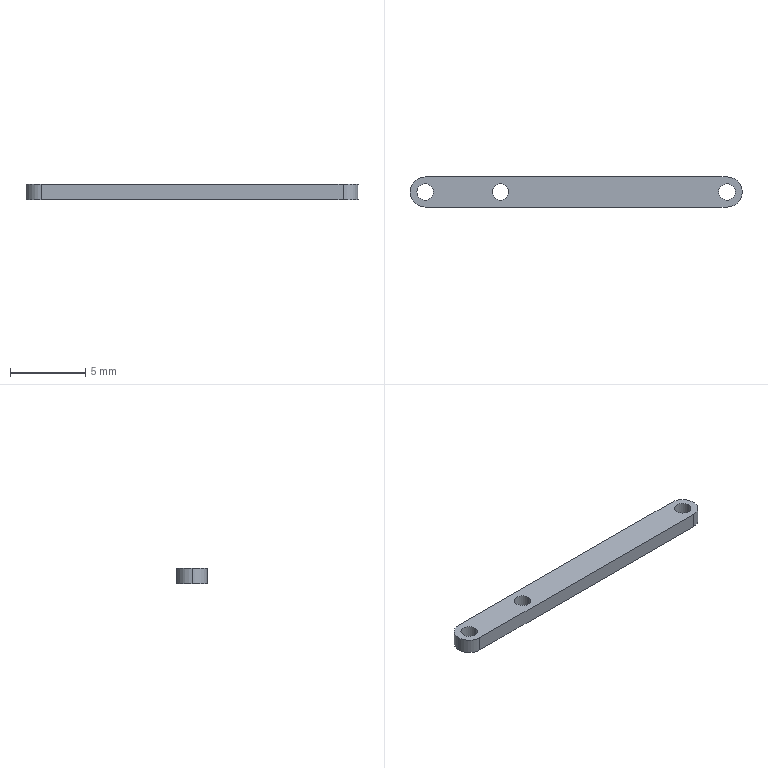Part | SolidWorks | features Extrusion 1, ICE 1 | 1 solid | 13 faces | box 22 x 2 x 1 mm | volume 40.291 mm3 | cylinder 9 | plane 4 | commonest cylinder face diameters 1.1 x6 2 x3
STEP:
#1=CARTESIAN_POINT('',(-5.55,0.,0.5));
#2=VERTEX_POINT('',#1);
#3=CARTESIAN_POINT('',(-4.45,0.,0.5));
#4=VERTEX_POINT('',#3);
#5=CARTESIAN_POINT('',(-5.,0.,0.5));
#6=DIRECTION('',(0.,0.,1.));
#7=DIRECTION('',(1.,0.,0.));
#8=AXIS2_PLACEMENT_3D('',#5,#6,#7);
#9=CIRCLE('',#8,0.55);
#10=EDGE_CURVE('',#2,#4,#9,.T.);
#11=ORIENTED_EDGE('',*,*,#10,.T.);
#12=CARTESIAN_POINT('',(-4.45,0.,-0.5));
#13=VERTEX_POINT('',#12);
#14=CARTESIAN_POINT('',(-4.45,0.,0.5));
#15=DIRECTION('',(0.,0.,-1.));
#16=VECTOR('',#15,1000.);
#17=LINE('',#14,#16);
#18=EDGE_CURVE('',#4,#13,#17,.T.);
#19=ORIENTED_EDGE('',*,*,#18,.T.);
#20=CARTESIAN_POINT('',(-5.55,0.,-0.5));
#21=VERTEX_POINT('',#20);
#22=CARTESIAN_POINT('',(-5.,0.,-0.5));
#23=DIRECTION('',(0.,0.,1.));
#24=DIRECTION('',(1.,0.,0.));
#25=AXIS2_PLACEMENT_3D('',#22,#23,#24);
#26=CIRCLE('',#25,0.55);
#27=EDGE_CURVE('',#21,#13,#26,.T.);
#28=ORIENTED_EDGE('',*,*,#27,.F.);
#29=CARTESIAN_POINT('',(-5.55,0.,0.5));
#30=DIRECTION('',(0.,0.,-1.));
#31=VECTOR('',#30,1000.);
#32=LINE('',#29,#31);
#33=EDGE_CURVE('',#2,#21,#32,.T.);
#34=ORIENTED_EDGE('',*,*,#33,.F.);
#35=EDGE_LOOP('',(#11,#19,#28,#34));
#36=FACE_OUTER_BOUND('',#35,.T.);
#37=CARTESIAN_POINT('',(-5.,0.,0.5));
#38=DIRECTION('',(0.,0.,-1.));
#39=DIRECTION('',(-1.,0.,0.));
#40=AXIS2_PLACEMENT_3D('',#37,#38,#39);
#41=CYLINDRICAL_SURFACE('',#40,0.55);
#42=ADVANCED_FACE('',(#36),#41,.F.);
#43=CARTESIAN_POINT('',(9.45,0.,0.5));
#44=VERTEX_POINT('',#43);
#45=CARTESIAN_POINT('',(10.55,0.,0.5));
#46=VERTEX_POINT('',#45);
#47=CARTESIAN_POINT('',(10.,0.,0.5));
#48=DIRECTION('',(0.,0.,1.));
#49=DIRECTION('',(1.,0.,0.));
#50=AXIS2_PLACEMENT_3D('',#47,#48,#49);
#51=CIRCLE('',#50,0.55);
#52=EDGE_CURVE('',#44,#46,#51,.T.);
#53=ORIENTED_EDGE('',*,*,#52,.T.);
#54=CARTESIAN_POINT('',(10.55,0.,-0.5));
#55=VERTEX_POINT('',#54);
#56=CARTESIAN_POINT('',(10.55,0.,0.5));
#57=DIRECTION('',(0.,0.,-1.));
#58=VECTOR('',#57,1000.);
#59=LINE('',#56,#58);
#60=EDGE_CURVE('',#46,#55,#59,.T.);
#61=ORIENTED_EDGE('',*,*,#60,.T.);
#62=CARTESIAN_POINT('',(9.45,0.,-0.5));
#63=VERTEX_POINT('',#62);
#64=CARTESIAN_POINT('',(10.,0.,-0.5));
#65=DIRECTION('',(0.,0.,1.));
#66=DIRECTION('',(1.,0.,0.));
#67=AXIS2_PLACEMENT_3D('',#64,#65,#66);
#68=CIRCLE('',#67,0.55);
#69=EDGE_CURVE('',#63,#55,#68,.T.);
#70=ORIENTED_EDGE('',*,*,#69,.F.);
#71=CARTESIAN_POINT('',(9.45,0.,0.5));
#72=DIRECTION('',(0.,0.,-1.));
#73=VECTOR('',#72,1000.);
#74=LINE('',#71,#73);
#75=EDGE_CURVE('',#44,#63,#74,.T.);
#76=ORIENTED_EDGE('',*,*,#75,.F.);
#77=EDGE_LOOP('',(#53,#61,#70,#76));
#78=FACE_OUTER_BOUND('',#77,.T.);
#79=CARTESIAN_POINT('',(10.,0.,0.5));
#80=DIRECTION('',(0.,0.,-1.));
#81=DIRECTION('',(-1.,0.,0.));
#82=AXIS2_PLACEMENT_3D('',#79,#80,#81);
#83=CYLINDRICAL_SURFACE('',#82,0.55);
#84=ADVANCED_FACE('',(#78),#83,.F.);
#85=CARTESIAN_POINT('',(-10.55,0.,0.5));
#86=VERTEX_POINT('',#85);
#87=CARTESIAN_POINT('',(-9.45,0.,0.5));
#88=VERTEX_POINT('',#87);
#89=CARTESIAN_POINT('',(-10.,0.,0.5));
#90=DIRECTION('',(0.,0.,1.));
#91=DIRECTION('',(1.,0.,0.));
#92=AXIS2_PLACEMENT_3D('',#89,#90,#91);
#93=CIRCLE('',#92,0.55);
#94=EDGE_CURVE('',#86,#88,#93,.T.);
#95=ORIENTED_EDGE('',*,*,#94,.T.);
#96=CARTESIAN_POINT('',(-9.45,0.,-0.5));
#97=VERTEX_POINT('',#96);
#98=CARTESIAN_POINT('',(-9.45,0.,0.5));
#99=DIRECTION('',(0.,0.,-1.));
#100=VECTOR('',#99,1000.);
#101=LINE('',#98,#100);
#102=EDGE_CURVE('',#88,#97,#101,.T.);
#103=ORIENTED_EDGE('',*,*,#102,.T.);
#104=CARTESIAN_POINT('',(-10.55,0.,-0.5));
#105=VERTEX_POINT('',#104);
#106=CARTESIAN_POINT('',(-10.,0.,-0.5));
#107=DIRECTION('',(0.,0.,1.));
#108=DIRECTION('',(1.,0.,0.));
#109=AXIS2_PLACEMENT_3D('',#106,#107,#108);
#110=CIRCLE('',#109,0.55);
#111=EDGE_CURVE('',#105,#97,#110,.T.);
#112=ORIENTED_EDGE('',*,*,#111,.F.);
#113=CARTESIAN_POINT('',(-10.55,0.,0.5));
#114=DIRECTION('',(0.,0.,-1.));
#115=VECTOR('',#114,1000.);
#116=LINE('',#113,#115);
#117=EDGE_CURVE('',#86,#105,#116,.T.);
#118=ORIENTED_EDGE('',*,*,#117,.F.);
#119=EDGE_LOOP('',(#95,#103,#112,#118));
#120=FACE_OUTER_BOUND('',#119,.T.);
#121=CARTESIAN_POINT('',(-10.,0.,0.5));
#122=DIRECTION('',(0.,0.,-1.));
#123=DIRECTION('',(-1.,0.,0.));
#124=AXIS2_PLACEMENT_3D('',#121,#122,#123);
#125=CYLINDRICAL_SURFACE('',#124,0.55);
#126=ADVANCED_FACE('',(#120),#125,.F.);
#127=CARTESIAN_POINT('',(-11.,0.,0.5));
#128=VERTEX_POINT('',#127);
#129=CARTESIAN_POINT('',(-10.,-1.,0.5));
#130=VERTEX_POINT('',#129);
#131=CARTESIAN_POINT('',(-10.,0.,0.5));
#132=DIRECTION('',(0.,0.,1.));
#133=DIRECTION('',(1.,0.,0.));
#134=AXIS2_PLACEMENT_3D('',#131,#132,#133);
#135=CIRCLE('',#134,1.);
#136=EDGE_CURVE('',#128,#130,#135,.T.);
#137=ORIENTED_EDGE('',*,*,#136,.F.);
#138=CARTESIAN_POINT('',(-11.,0.,-0.5));
#139=VERTEX_POINT('',#138);
#140=CARTESIAN_POINT('',(-11.,0.,0.5));
#141=DIRECTION('',(0.,0.,-1.));
#142=VECTOR('',#141,1000.);
#143=LINE('',#140,#142);
#144=EDGE_CURVE('',#128,#139,#143,.T.);
#145=ORIENTED_EDGE('',*,*,#144,.T.);
#146=CARTESIAN_POINT('',(-10.,-1.,-0.5));
#147=VERTEX_POINT('',#146);
#148=CARTESIAN_POINT('',(-10.,0.,-0.5));
#149=DIRECTION('',(0.,0.,1.));
#150=DIRECTION('',(1.,0.,0.));
#151=AXIS2_PLACEMENT_3D('',#148,#149,#150);
#152=CIRCLE('',#151,1.);
#153=EDGE_CURVE('',#139,#147,#152,.T.);
#154=ORIENTED_EDGE('',*,*,#153,.T.);
#155=CARTESIAN_POINT('',(-10.,-1.,0.5));
#156=DIRECTION('',(0.,0.,-1.));
#157=VECTOR('',#156,1000.);
#158=LINE('',#155,#157);
#159=EDGE_CURVE('',#130,#147,#158,.T.);
#160=ORIENTED_EDGE('',*,*,#159,.F.);
#161=EDGE_LOOP('',(#137,#145,#154,#160));
#162=FACE_OUTER_BOUND('',#161,.T.);
#163=CARTESIAN_POINT('',(-10.,0.,0.5));
#164=DIRECTION('',(0.,0.,-1.));
#165=DIRECTION('',(-1.,0.,0.));
#166=AXIS2_PLACEMENT_3D('',#163,#164,#165);
#167=CYLINDRICAL_SURFACE('',#166,1.);
#168=ADVANCED_FACE('',(#162),#167,.T.);
#169=ORIENTED_EDGE('',*,*,#52,.F.);
#170=CARTESIAN_POINT('',(10.,0.,0.5));
#171=DIRECTION('',(0.,0.,1.));
#172=DIRECTION('',(1.,0.,0.));
#173=AXIS2_PLACEMENT_3D('',#170,#171,#172);
#174=CIRCLE('',#173,0.55);
#175=EDGE_CURVE('',#46,#44,#174,.T.);
#176=ORIENTED_EDGE('',*,*,#175,.F.);
#177=EDGE_LOOP('',(#169,#176));
#178=FACE_BOUND('',#177,.T.);
#179=CARTESIAN_POINT('',(-10.,1.,0.5));
#180=VERTEX_POINT('',#179);
#181=CARTESIAN_POINT('',(-10.,0.,0.5));
#182=DIRECTION('',(0.,0.,1.));
#183=DIRECTION('',(1.,0.,0.));
#184=AXIS2_PLACEMENT_3D('',#181,#182,#183);
#185=CIRCLE('',#184,1.);
#186=EDGE_CURVE('',#180,#128,#185,.T.);
#187=ORIENTED_EDGE('',*,*,#186,.T.);
#188=ORIENTED_EDGE('',*,*,#136,.T.);
#189=CARTESIAN_POINT('',(10.,-1.,0.5));
#190=VERTEX_POINT('',#189);
#191=CARTESIAN_POINT('',(-10.,-1.,0.5));
#192=DIRECTION('',(1.,0.,0.));
#193=VECTOR('',#192,1000.);
#194=LINE('',#191,#193);
#195=EDGE_CURVE('',#130,#190,#194,.T.);
#196=ORIENTED_EDGE('',*,*,#195,.T.);
#197=CARTESIAN_POINT('',(10.,1.,0.5));
#198=VERTEX_POINT('',#197);
#199=CARTESIAN_POINT('',(10.,0.,0.5));
#200=DIRECTION('',(0.,0.,1.));
#201=DIRECTION('',(1.,0.,0.));
#202=AXIS2_PLACEMENT_3D('',#199,#200,#201);
#203=CIRCLE('',#202,1.);
#204=EDGE_CURVE('',#190,#198,#203,.T.);
#205=ORIENTED_EDGE('',*,*,#204,.T.);
#206=CARTESIAN_POINT('',(-10.,1.,0.5));
#207=DIRECTION('',(-1.,0.,0.));
#208=VECTOR('',#207,1000.);
#209=LINE('',#206,#208);
#210=EDGE_CURVE('',#198,#180,#209,.T.);
#211=ORIENTED_EDGE('',*,*,#210,.T.);
#212=EDGE_LOOP('',(#187,#188,#196,#205,#211));
#213=FACE_OUTER_BOUND('',#212,.T.);
#214=ORIENTED_EDGE('',*,*,#94,.F.);
#215=CARTESIAN_POINT('',(-10.,0.,0.5));
#216=DIRECTION('',(0.,0.,1.));
#217=DIRECTION('',(1.,0.,0.));
#218=AXIS2_PLACEMENT_3D('',#215,#216,#217);
#219=CIRCLE('',#218,0.55);
#220=EDGE_CURVE('',#88,#86,#219,.T.);
#221=ORIENTED_EDGE('',*,*,#220,.F.);
#222=EDGE_LOOP('',(#214,#221));
#223=FACE_BOUND('',#222,.T.);
#224=ORIENTED_EDGE('',*,*,#10,.F.);
#225=CARTESIAN_POINT('',(-5.,0.,0.5));
#226=DIRECTION('',(0.,0.,1.));
#227=DIRECTION('',(1.,0.,0.));
#228=AXIS2_PLACEMENT_3D('',#225,#226,#227);
#229=CIRCLE('',#228,0.55);
#230=EDGE_CURVE('',#4,#2,#229,.T.);
#231=ORIENTED_EDGE('',*,*,#230,.F.);
#232=EDGE_LOOP('',(#224,#231));
#233=FACE_BOUND('',#232,.T.);
#234=CARTESIAN_POINT('',(-10.,0.,0.5));
#235=DIRECTION('',(0.,0.,1.));
#236=DIRECTION('',(1.,0.,0.));
#237=AXIS2_PLACEMENT_3D('',#234,#235,#236);
#238=PLANE('',#237);
#239=ADVANCED_FACE('',(#178,#213,#223,#233),#238,.T.);
#240=CARTESIAN_POINT('',(-10.,1.,-0.5));
#241=VERTEX_POINT('',#240);
#242=CARTESIAN_POINT('',(-10.,0.,-0.5));
#243=DIRECTION('',(0.,0.,1.));
#244=DIRECTION('',(1.,0.,0.));
#245=AXIS2_PLACEMENT_3D('',#242,#243,#244);
#246=CIRCLE('',#245,1.);
#247=EDGE_CURVE('',#241,#139,#246,.T.);
#248=ORIENTED_EDGE('',*,*,#247,.F.);
#249=CARTESIAN_POINT('',(10.,1.,-0.5));
#250=VERTEX_POINT('',#249);
#251=CARTESIAN_POINT('',(-10.,1.,-0.5));
#252=DIRECTION('',(-1.,0.,0.));
#253=VECTOR('',#252,1000.);
#254=LINE('',#251,#253);
#255=EDGE_CURVE('',#250,#241,#254,.T.);
#256=ORIENTED_EDGE('',*,*,#255,.F.);
#257=CARTESIAN_POINT('',(10.,-1.,-0.5));
#258=VERTEX_POINT('',#257);
#259=CARTESIAN_POINT('',(10.,0.,-0.5));
#260=DIRECTION('',(0.,0.,1.));
#261=DIRECTION('',(1.,0.,0.));
#262=AXIS2_PLACEMENT_3D('',#259,#260,#261);
#263=CIRCLE('',#262,1.);
#264=EDGE_CURVE('',#258,#250,#263,.T.);
#265=ORIENTED_EDGE('',*,*,#264,.F.);
#266=CARTESIAN_POINT('',(-10.,-1.,-0.5));
#267=DIRECTION('',(1.,0.,0.));
#268=VECTOR('',#267,1000.);
#269=LINE('',#266,#268);
#270=EDGE_CURVE('',#147,#258,#269,.T.);
#271=ORIENTED_EDGE('',*,*,#270,.F.);
#272=ORIENTED_EDGE('',*,*,#153,.F.);
#273=EDGE_LOOP('',(#248,#256,#265,#271,#272));
#274=FACE_OUTER_BOUND('',#273,.T.);
#275=ORIENTED_EDGE('',*,*,#111,.T.);
#276=CARTESIAN_POINT('',(-10.,0.,-0.5));
#277=DIRECTION('',(0.,0.,1.));
#278=DIRECTION('',(1.,0.,0.));
#279=AXIS2_PLACEMENT_3D('',#276,#277,#278);
#280=CIRCLE('',#279,0.55);
#281=EDGE_CURVE('',#97,#105,#280,.T.);
#282=ORIENTED_EDGE('',*,*,#281,.T.);
#283=EDGE_LOOP('',(#275,#282));
#284=FACE_BOUND('',#283,.T.);
#285=ORIENTED_EDGE('',*,*,#69,.T.);
#286=CARTESIAN_POINT('',(10.,0.,-0.5));
#287=DIRECTION('',(0.,0.,1.));
#288=DIRECTION('',(1.,0.,0.));
#289=AXIS2_PLACEMENT_3D('',#286,#287,#288);
#290=CIRCLE('',#289,0.55);
#291=EDGE_CURVE('',#55,#63,#290,.T.);
#292=ORIENTED_EDGE('',*,*,#291,.T.);
#293=EDGE_LOOP('',(#285,#292));
#294=FACE_BOUND('',#293,.T.);
#295=ORIENTED_EDGE('',*,*,#27,.T.);
#296=CARTESIAN_POINT('',(-5.,0.,-0.5));
#297=DIRECTION('',(0.,0.,1.));
#298=DIRECTION('',(1.,0.,0.));
#299=AXIS2_PLACEMENT_3D('',#296,#297,#298);
#300=CIRCLE('',#299,0.55);
#301=EDGE_CURVE('',#13,#21,#300,.T.);
#302=ORIENTED_EDGE('',*,*,#301,.T.);
#303=EDGE_LOOP('',(#295,#302));
#304=FACE_BOUND('',#303,.T.);
#305=CARTESIAN_POINT('',(-10.,0.,-0.5));
#306=DIRECTION('',(0.,0.,1.));
#307=DIRECTION('',(1.,0.,0.));
#308=AXIS2_PLACEMENT_3D('',#305,#306,#307);
#309=PLANE('',#308);
#310=ADVANCED_FACE('',(#274,#284,#294,#304),#309,.F.);
#311=ORIENTED_EDGE('',*,*,#144,.F.);
#312=ORIENTED_EDGE('',*,*,#186,.F.);
#313=CARTESIAN_POINT('',(-10.,1.,0.5));
#314=DIRECTION('',(0.,0.,-1.));
#315=VECTOR('',#314,1000.);
#316=LINE('',#313,#315);
#317=EDGE_CURVE('',#180,#241,#316,.T.);
#318=ORIENTED_EDGE('',*,*,#317,.T.);
#319=ORIENTED_EDGE('',*,*,#247,.T.);
#320=EDGE_LOOP('',(#311,#312,#318,#319));
#321=FACE_OUTER_BOUND('',#320,.T.);
#322=CARTESIAN_POINT('',(-10.,0.,0.5));
#323=DIRECTION('',(0.,0.,-1.));
#324=DIRECTION('',(-1.,0.,0.));
#325=AXIS2_PLACEMENT_3D('',#322,#323,#324);
#326=CYLINDRICAL_SURFACE('',#325,1.);
#327=ADVANCED_FACE('',(#321),#326,.T.);
#328=ORIENTED_EDGE('',*,*,#270,.T.);
#329=CARTESIAN_POINT('',(10.,-1.,0.5));
#330=DIRECTION('',(0.,0.,-1.));
#331=VECTOR('',#330,1000.);
#332=LINE('',#329,#331);
#333=EDGE_CURVE('',#190,#258,#332,.T.);
#334=ORIENTED_EDGE('',*,*,#333,.F.);
#335=ORIENTED_EDGE('',*,*,#195,.F.);
#336=ORIENTED_EDGE('',*,*,#159,.T.);
#337=EDGE_LOOP('',(#328,#334,#335,#336));
#338=FACE_OUTER_BOUND('',#337,.T.);
#339=CARTESIAN_POINT('',(-10.,-1.,0.5));
#340=DIRECTION('',(0.,1.,0.));
#341=DIRECTION('',(-1.,0.,0.));
#342=AXIS2_PLACEMENT_3D('',#339,#340,#341);
#343=PLANE('',#342);
#344=ADVANCED_FACE('',(#338),#343,.F.);
#345=ORIENTED_EDGE('',*,*,#264,.T.);
#346=CARTESIAN_POINT('',(10.,1.,0.5));
#347=DIRECTION('',(0.,0.,-1.));
#348=VECTOR('',#347,1000.);
#349=LINE('',#346,#348);
#350=EDGE_CURVE('',#198,#250,#349,.T.);
#351=ORIENTED_EDGE('',*,*,#350,.F.);
#352=ORIENTED_EDGE('',*,*,#204,.F.);
#353=ORIENTED_EDGE('',*,*,#333,.T.);
#354=EDGE_LOOP('',(#345,#351,#352,#353));
#355=FACE_OUTER_BOUND('',#354,.T.);
#356=CARTESIAN_POINT('',(10.,0.,0.5));
#357=DIRECTION('',(0.,0.,-1.));
#358=DIRECTION('',(-1.,0.,0.));
#359=AXIS2_PLACEMENT_3D('',#356,#357,#358);
#360=CYLINDRICAL_SURFACE('',#359,1.);
#361=ADVANCED_FACE('',(#355),#360,.T.);
#362=ORIENTED_EDGE('',*,*,#255,.T.);
#363=ORIENTED_EDGE('',*,*,#317,.F.);
#364=ORIENTED_EDGE('',*,*,#210,.F.);
#365=ORIENTED_EDGE('',*,*,#350,.T.);
#366=EDGE_LOOP('',(#362,#363,#364,#365));
#367=FACE_OUTER_BOUND('',#366,.T.);
#368=CARTESIAN_POINT('',(-10.,1.,0.5));
#369=DIRECTION('',(0.,-1.,0.));
#370=DIRECTION('',(1.,0.,0.));
#371=AXIS2_PLACEMENT_3D('',#368,#369,#370);
#372=PLANE('',#371);
#373=ADVANCED_FACE('',(#367),#372,.F.);
#374=ORIENTED_EDGE('',*,*,#102,.F.);
#375=ORIENTED_EDGE('',*,*,#220,.T.);
#376=ORIENTED_EDGE('',*,*,#117,.T.);
#377=ORIENTED_EDGE('',*,*,#281,.F.);
#378=EDGE_LOOP('',(#374,#375,#376,#377));
#379=FACE_OUTER_BOUND('',#378,.T.);
#380=CARTESIAN_POINT('',(-10.,0.,0.5));
#381=DIRECTION('',(0.,0.,-1.));
#382=DIRECTION('',(-1.,0.,0.));
#383=AXIS2_PLACEMENT_3D('',#380,#381,#382);
#384=CYLINDRICAL_SURFACE('',#383,0.55);
#385=ADVANCED_FACE('',(#379),#384,.F.);
#386=ORIENTED_EDGE('',*,*,#60,.F.);
#387=ORIENTED_EDGE('',*,*,#175,.T.);
#388=ORIENTED_EDGE('',*,*,#75,.T.);
#389=ORIENTED_EDGE('',*,*,#291,.F.);
#390=EDGE_LOOP('',(#386,#387,#388,#389));
#391=FACE_OUTER_BOUND('',#390,.T.);
#392=CARTESIAN_POINT('',(10.,0.,0.5));
#393=DIRECTION('',(0.,0.,-1.));
#394=DIRECTION('',(-1.,0.,0.));
#395=AXIS2_PLACEMENT_3D('',#392,#393,#394);
#396=CYLINDRICAL_SURFACE('',#395,0.55);
#397=ADVANCED_FACE('',(#391),#396,.F.);
#398=ORIENTED_EDGE('',*,*,#18,.F.);
#399=ORIENTED_EDGE('',*,*,#230,.T.);
#400=ORIENTED_EDGE('',*,*,#33,.T.);
#401=ORIENTED_EDGE('',*,*,#301,.F.);
#402=EDGE_LOOP('',(#398,#399,#400,#401));
#403=FACE_OUTER_BOUND('',#402,.T.);
#404=CARTESIAN_POINT('',(-5.,0.,0.5));
#405=DIRECTION('',(0.,0.,-1.));
#406=DIRECTION('',(-1.,0.,0.));
#407=AXIS2_PLACEMENT_3D('',#404,#405,#406);
#408=CYLINDRICAL_SURFACE('',#407,0.55);
#409=ADVANCED_FACE('',(#403),#408,.F.);
#410=CLOSED_SHELL('',(#42,#84,#126,#168,#239,#310,#327,#344,#361,#373,#385,#397,#409));
#411=MANIFOLD_SOLID_BREP('',#410);
#412=CARTESIAN_POINT('',(0.,0.,0.));
#413=DIRECTION('',(0.,0.,1.));
#414=DIRECTION('',(1.,0.,0.));
#415=AXIS2_PLACEMENT_3D('',#412,#413,#414);
#416=(LENGTH_UNIT()NAMED_UNIT(*)SI_UNIT(.MILLI.,.METRE.));
#417=UNCERTAINTY_MEASURE_WITH_UNIT(LENGTH_MEASURE(0.00001),#416,'','');
#418=(NAMED_UNIT(*)PLANE_ANGLE_UNIT()SI_UNIT($,.RADIAN.));
#419=(NAMED_UNIT(*)SI_UNIT($,.STERADIAN.)SOLID_ANGLE_UNIT());
#420=(GEOMETRIC_REPRESENTATION_CONTEXT(3)GLOBAL_UNCERTAINTY_ASSIGNED_CONTEXT((#417))GLOBAL_UNIT_ASSIGNED_CONTEXT((#416,#418,#419))REPRESENTATION_CONTEXT('',''));
#421=ADVANCED_BREP_SHAPE_REPRESENTATION('',(#411,#415),#420);